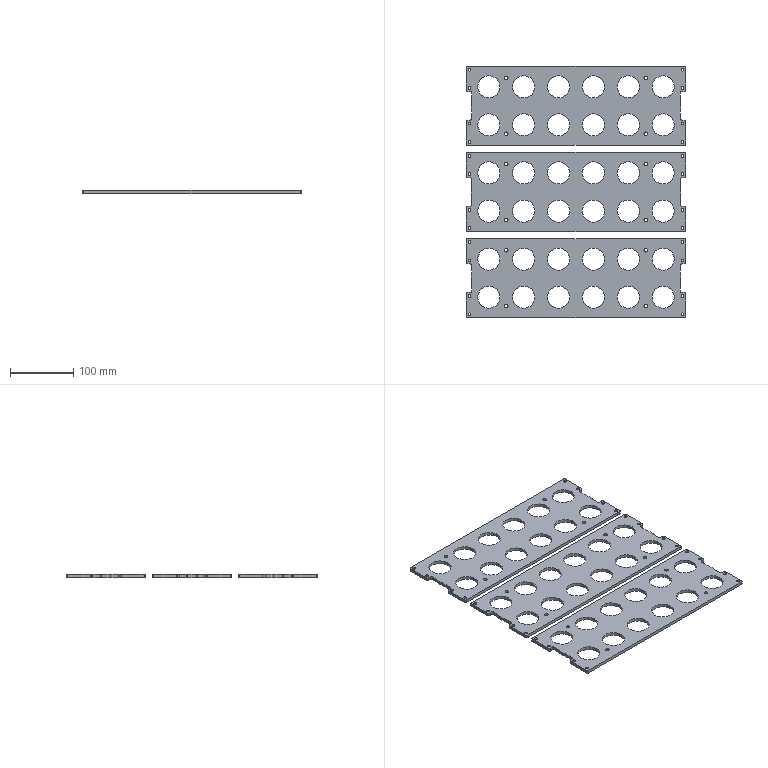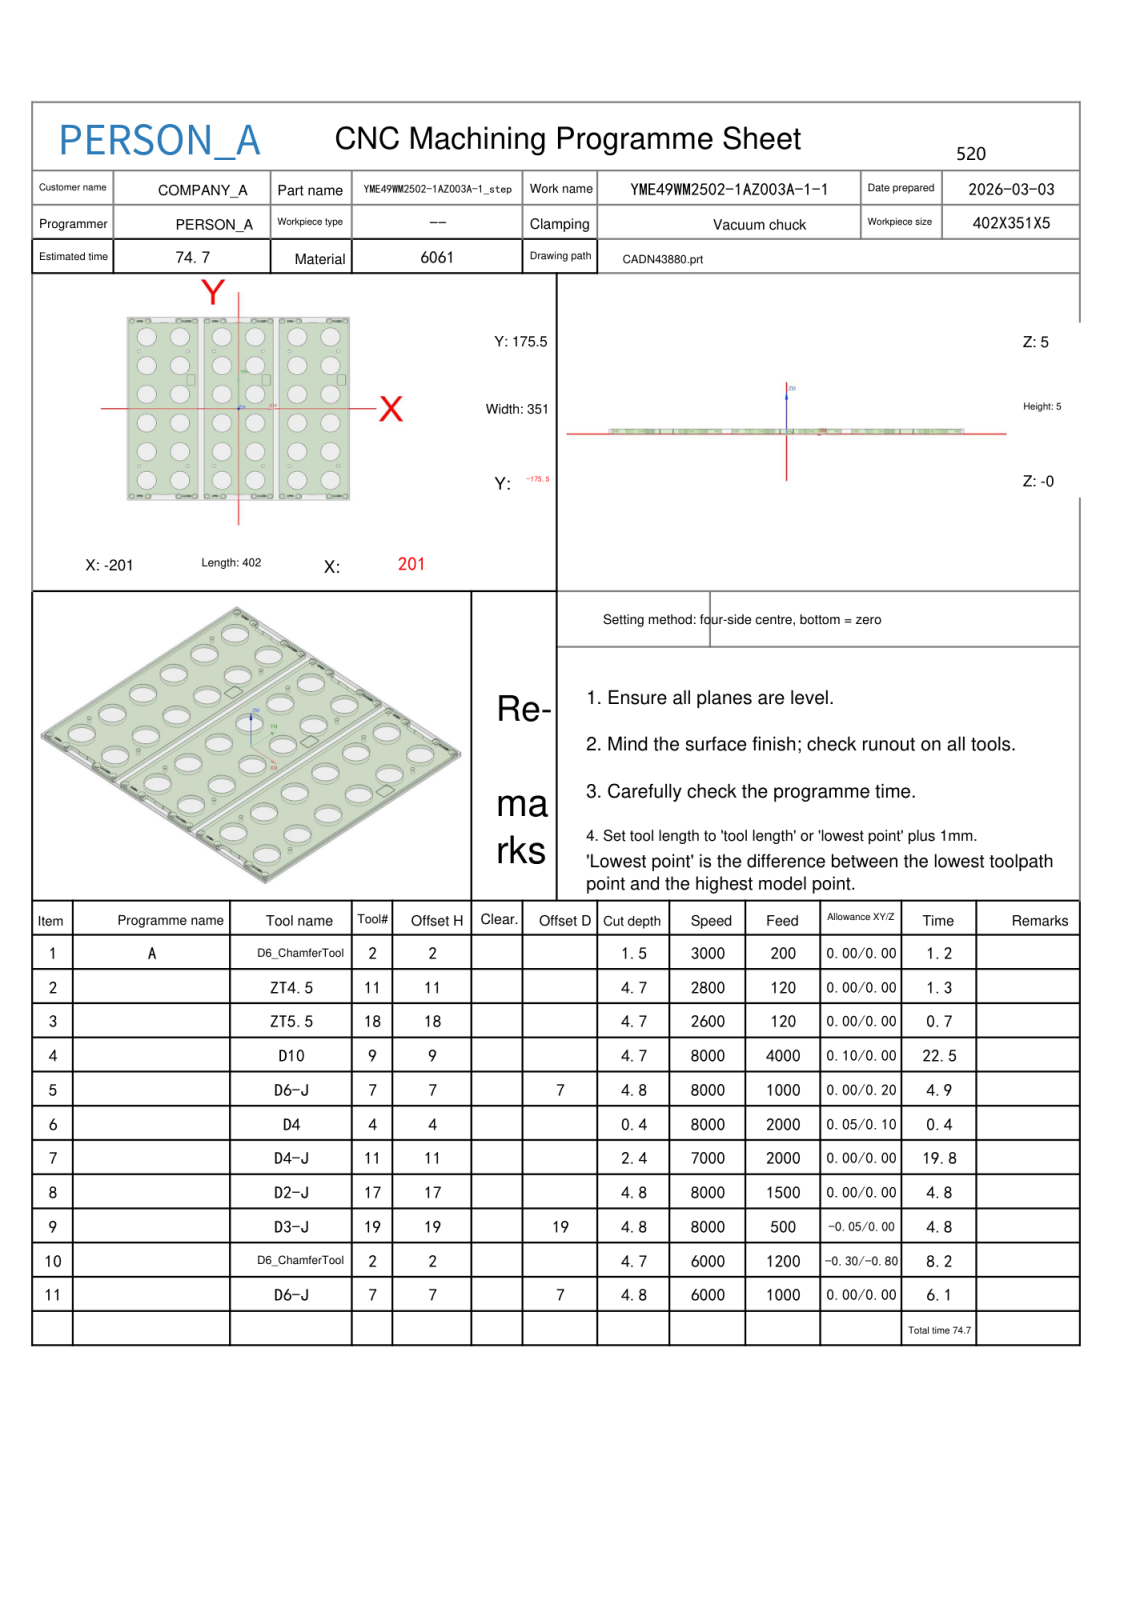NC program | NX | posted by the shop | part box 346 x 397 x 5 mm
Lines 4965 to 5785 of 51232:
N7 T11 M06
(D4-J  D=4. R=0. H=11 ce=0.00 di=0.00)
G00 G90 G54 X-192.342 Y-170.608 M03 S7000
G43 H11 Z35.
M08
Z6.5
G01 X-191.943 Y-170.475 Z6.478 F2000.
X-191.558 Y-170.272 Z6.455
X-191.211 Y-170.01 Z6.432
X-190.91 Y-169.695 Z6.41
X-190.665 Y-169.337 Z6.387
X-190.48 Y-168.943 Z6.364
X-190.384 Y-168.629 Z6.347
X-190.317 Y-168.201 Z6.324
X-190.319 Y-167.767 Z6.301
X-190.367 Y-167.443 Z6.284
X-190.497 Y-167.012 Z6.261
X-190.697 Y-166.608 Z6.237
X-190.961 Y-166.244 Z6.213
X-191.282 Y-165.929 Z6.19
X-191.652 Y-165.671 Z6.166
X-192.059 Y-165.479 Z6.143
X-192.492 Y-165.358 Z6.119
X-192.94 Y-165.31 Z6.095
X-193.389 Y-165.337 Z6.072
X-193.827 Y-165.439 Z6.048
X-194.242 Y-165.613 Z6.025
X-194.523 Y-165.782 Z6.008
X-194.84 Y-166.037 Z5.986
X-195.115 Y-166.337 Z5.965
X-195.342 Y-166.675 Z5.944
X-195.515 Y-167.043 Z5.922
X-195.63 Y-167.433 Z5.901
X-195.686 Y-167.836 Z5.88
Y-168.164 Z5.862
X-195.623 Y-168.601 Z5.839
X-195.49 Y-169.021 Z5.816
X-195.289 Y-169.414 Z5.793
X-195.027 Y-169.769 Z5.77
X-194.711 Y-170.077 Z5.747
X-194.446 Y-170.27 Z5.73
X-194.061 Y-170.473 Z5.707
X-193.649 Y-170.611 Z5.684
X-193.22 Y-170.682 Z5.661
X-192.785 Z5.638
X-192.355 Y-170.613 Z5.616
X-191.943 Y-170.475 Z5.593
X-191.558 Y-170.272 Z5.57
X-191.211 Y-170.01 Z5.547
X-190.91 Y-169.695 Z5.524
X-190.665 Y-169.337 Z5.502
X-190.48 Y-168.943 Z5.479
X-190.384 Y-168.629 Z5.462
X-190.317 Y-168.201 Z5.439
X-190.319 Y-167.767 Z5.416
X-190.367 Y-167.443 Z5.399
X-190.497 Y-167.012 Z5.375
X-190.697 Y-166.608 Z5.352
X-190.961 Y-166.244 Z5.328
X-191.282 Y-165.929 Z5.305
X-191.652 Y-165.671 Z5.281
X-192.059 Y-165.479 Z5.258
X-192.492 Y-165.358 Z5.234
X-192.94 Y-165.31 Z5.21
X-193.389 Y-165.337 Z5.187
X-193.827 Y-165.439 Z5.163
X-194.242 Y-165.613 Z5.14
X-194.523 Y-165.782 Z5.122
X-194.84 Y-166.037 Z5.101
X-195.115 Y-166.337 Z5.08
X-195.342 Y-166.675 Z5.058
X-195.515 Y-167.043 Z5.037
X-195.63 Y-167.433 Z5.016
X-195.686 Y-167.836 Z4.994
Y-168. Z4.986
G03 X-193. Y-170.686 I2.686 J0.0
X-190.314 Y-168. I0.0 J2.686
X-193. Y-165.314 I-2.686 J0.0
X-195.686 Y-168. I0.0 J-2.686
G01 X-195.678 Y-168.08 Z4.979
X-195.667 Y-168.161 Z4.972
G03 X-193. Y-170.672 I2.667 J.161
X-190.328 Y-168. I0.0 J2.672
X-193. Y-165.328 I-2.672 J0.0
X-195.672 Y-168. I0.0 J-2.672
G01 X-195.663 Y-168.08 Z4.965
X-195.653 Y-168.161 Z4.958
G03 X-193. Y-170.658 I2.653 J.161
X-190.342 Y-168. I0.0 J2.658
X-193. Y-165.342 I-2.658 J0.0
X-195.658 Y-168. I0.0 J-2.658
G01 X-195.649 Y-168.08 Z4.951
X-195.639 Y-168.161 Z4.943
G03 X-193. Y-170.643 I2.639 J.161
X-190.357 Y-168. I0.0 J2.643
X-193. Y-165.357 I-2.643 J0.0
X-195.643 Y-168. I0.0 J-2.643
G01 X-195.635 Y-168.08 Z4.936
X-195.624 Y-168.161 Z4.929
G03 X-193. Y-170.629 I2.624 J.161
X-190.371 Y-168. I0.0 J2.629
X-193. Y-165.371 I-2.629 J0.0
X-195.629 Y-168. I0.0 J-2.629
G01 X-195.621 Y-168.08 Z4.922
X-195.61 Y-168.161 Z4.915
G03 X-193. Y-170.615 I2.61 J.161
X-190.385 Y-168. I0.0 J2.615
X-193. Y-165.385 I-2.615 J0.0
X-195.615 Y-168. I0.0 J-2.615
G01 X-195.607 Y-168.08 Z4.908
X-195.596 Y-168.161 Z4.901
G03 X-193. Y-170.601 I2.596 J.161
X-190.399 Y-168. I0.0 J2.601
X-193. Y-165.399 I-2.601 J0.0
X-195.601 Y-168. I0.0 J-2.601
G01 X-195.593 Y-168.08 Z4.894
X-195.582 Y-168.161 Z4.887
G03 X-193. Y-170.587 I2.582 J.161
X-190.413 Y-168. I0.0 J2.587
X-193. Y-165.413 I-2.587 J0.0
X-195.587 Y-168. I0.0 J-2.587
G01 X-195.579 Y-168.08 Z4.88
X-195.568 Y-168.161 Z4.873
G03 X-193. Y-170.573 I2.568 J.161
X-190.427 Y-168. I0.0 J2.573
X-193. Y-165.427 I-2.573 J0.0
X-195.573 Y-168. I0.0 J-2.573
G01 X-195.564 Y-168.08 Z4.866
X-195.554 Y-168.161 Z4.859
G03 X-193. Y-170.559 I2.554 J.161
X-190.441 Y-168. I0.0 J2.559
X-193. Y-165.441 I-2.559 J0.0
X-195.559 Y-168. I0.0 J-2.559
G01 X-195.55 Y-168.08 Z4.852
X-195.539 Y-168.161 Z4.844
G03 X-193. Y-170.544 I2.539 J.161
X-190.456 Y-168. I0.0 J2.544
X-193. Y-165.456 I-2.544 J0.0
X-195.544 Y-168. I0.0 J-2.544
G01 X-195.536 Y-168.08 Z4.837
X-195.525 Y-168.161 Z4.83
G03 X-193. Y-170.53 I2.525 J.161
X-190.47 Y-168. I0.0 J2.53
X-193. Y-165.47 I-2.53 J0.0
X-195.53 Y-168. I0.0 J-2.53
G01 X-195.522 Y-168.08 Z4.823
X-195.511 Y-168.161 Z4.816
G03 X-193. Y-170.516 I2.511 J.161
X-190.484 Y-168. I0.0 J2.516
X-193. Y-165.484 I-2.516 J0.0
X-195.516 Y-168. I0.0 J-2.516
G01 X-195.508 Y-168.08 Z4.809
X-195.497 Y-168.161 Z4.802
G03 X-193. Y-170.503 I2.497 J.161
X-190.498 Y-168. I0.0 J2.502
X-193. Y-165.498 I-2.502 J0.0
X-195.503 Y-168. I0.0 J-2.502
G01 X-195.494 Y-168.08 Z4.795
X-195.483 Y-168.161 Z4.788
G03 X-193. Y-170.488 I2.483 J.161
X-190.512 Y-168. I0.0 J2.488
X-193. Y-165.512 I-2.488 J0.0
X-195.488 Y-168. I0.0 J-2.488
G01 X-195.479 Y-168.08 Z4.781
X-195.469 Y-168.161 Z4.774
G03 X-193. Y-170.474 I2.469 J.161
X-190.526 Y-168. I0.0 J2.474
X-193. Y-165.526 I-2.474 J0.0
X-195.474 Y-168. I0.0 J-2.474
G01 X-195.465 Y-168.08 Z4.767
X-195.454 Y-168.161 Z4.76
G03 X-193. Y-170.46 I2.454 J.161
X-190.54 Y-168. I0.0 J2.46
X-193. Y-165.54 I-2.46 J0.0
X-195.46 Y-168. I0.0 J-2.46
G01 X-195.451 Y-168.08 Z4.753
X-195.44 Y-168.161 Z4.745
G03 X-193. Y-170.445 I2.44 J.161
X-190.555 Y-168. I0.0 J2.445
X-193. Y-165.555 I-2.445 J0.0
X-195.445 Y-168. I0.0 J-2.445
G01 X-195.437 Y-168.08 Z4.738
X-195.426 Y-168.161 Z4.731
G03 X-193. Y-170.431 I2.426 J.161
X-190.569 Y-168. I0.0 J2.431
X-193. Y-165.569 I-2.431 J0.0
X-195.431 Y-168. I0.0 J-2.431
G01 X-195.423 Y-168.08 Z4.724
X-195.412 Y-168.161 Z4.717
G03 X-193. Y-170.417 I2.412 J.161
X-190.583 Y-168. I0.0 J2.417
X-193. Y-165.583 I-2.417 J0.0
X-195.417 Y-168. I0.0 J-2.417
G01 X-195.409 Y-168.08 Z4.71
X-195.398 Y-168.161 Z4.703
G03 X-193. Y-170.403 I2.398 J.161
X-190.597 Y-168. I0.0 J2.403
X-193. Y-165.597 I-2.403 J0.0
X-195.403 Y-168. I0.0 J-2.403
G01 X-195.395 Y-168.08 Z4.696
X-195.383 Y-168.161 Z4.689
G03 X-193. Y-170.389 I2.383 J.161
X-190.611 Y-168. I0.0 J2.389
X-193. Y-165.611 I-2.389 J0.0
X-195.389 Y-168. I0.0 J-2.389
G01 X-195.38 Y-168.08 Z4.682
X-195.369 Y-168.161 Z4.675
G03 X-193. Y-170.375 I2.369 J.161
X-190.625 Y-168. I0.0 J2.375
X-193. Y-165.625 I-2.375 J0.0
X-195.375 Y-168. I0.0 J-2.375
G01 X-195.366 Y-168.08 Z4.668
X-195.355 Y-168.161 Z4.661
G03 X-193. Y-170.361 I2.355 J.161
X-190.639 Y-168. I0.0 J2.361
X-193. Y-165.639 I-2.361 J0.0
X-195.361 Y-168. I0.0 J-2.361
G01 X-195.352 Y-168.08 Z4.654
X-195.341 Y-168.161 Z4.646
G03 X-193. Y-170.346 I2.341 J.161
X-190.654 Y-168. I0.0 J2.346
X-193. Y-165.654 I-2.346 J0.0
X-195.346 Y-168. I0.0 J-2.346
G01 X-195.338 Y-168.08 Z4.639
X-195.327 Y-168.161 Z4.632
G03 X-193. Y-170.332 I2.327 J.161
X-190.668 Y-168. I0.0 J2.332
X-193. Y-165.668 I-2.332 J0.0
X-195.332 Y-168. I0.0 J-2.332
G01 X-195.324 Y-168.08 Z4.625
X-195.313 Y-168.161 Z4.618
G03 X-193. Y-170.318 I2.313 J.161
X-190.682 Y-168. I0.0 J2.318
X-193. Y-165.682 I-2.318 J0.0
X-195.318 Y-168. I0.0 J-2.318
G01 X-195.31 Y-168.08 Z4.611
X-195.298 Y-168.161 Z4.604
G03 X-193. Y-170.304 I2.298 J.161
X-190.696 Y-168. I0.0 J2.304
X-193. Y-165.696 I-2.304 J0.0
X-195.304 Y-168. I0.0 J-2.304
G01 X-195.296 Y-168.08 Z4.597
X-195.284 Y-168.161 Z4.59
G03 X-193. Y-170.29 I2.284 J.161
X-190.71 Y-168. I0.0 J2.29
X-193. Y-165.71 I-2.29 J0.0
X-195.29 Y-168. I0.0 J-2.29
G01 X-195.281 Y-168.08 Z4.583
X-195.27 Y-168.161 Z4.576
G03 X-193. Y-170.276 I2.27 J.161
X-190.724 Y-168. I0.0 J2.276
X-193. Y-165.724 I-2.276 J0.0
X-195.276 Y-168. I0.0 J-2.276
G01 X-195.267 Y-168.08 Z4.569
X-195.256 Y-168.161 Z4.562
G03 X-193. Y-170.262 I2.256 J.161
X-190.738 Y-168. I0.0 J2.262
X-193. Y-165.738 I-2.262 J0.0
X-195.262 Y-168. I0.0 J-2.262
G01 X-195.253 Y-168.08 Z4.555
X-195.242 Y-168.16 Z4.547
G03 X-193. Y-170.247 I2.242 J.16
X-190.753 Y-168. I0.0 J2.247
X-193. Y-165.753 I-2.247 J0.0
X-195.247 Y-168. I0.0 J-2.247
G01 X-195.239 Y-168.08 Z4.54
X-195.228 Y-168.16 Z4.533
G03 X-193. Y-170.233 I2.228 J.16
X-190.767 Y-168. I0.0 J2.233
X-193. Y-165.767 I-2.233 J0.0
X-195.233 Y-168. I0.0 J-2.233
G01 X-195.225 Y-168.08 Z4.526
X-195.213 Y-168.16 Z4.519
G03 X-193. Y-170.219 I2.213 J.16
X-190.781 Y-168. I0.0 J2.219
X-193. Y-165.781 I-2.219 J0.0
X-195.219 Y-168. I0.0 J-2.219
G01 X-195.211 Y-168.08 Z4.512
X-195.199 Y-168.16 Z4.505
G03 X-193. Y-170.205 I2.199 J.16
X-190.795 Y-168. I0.0 J2.205
X-193. Y-165.795 I-2.205 J0.0
X-195.205 Y-168. I0.0 J-2.205
G01 X-195.196 Y-168.08 Z4.498
X-195.185 Y-168.16 Z4.491
G03 X-193. Y-170.191 I2.185 J.16
X-190.809 Y-168. I0.0 J2.191
X-193. Y-165.809 I-2.191 J0.0
X-195.191 Y-168. I0.0 J-2.191
G01 X-195.182 Y-168.08 Z4.484
X-195.171 Y-168.16 Z4.477
G03 X-193. Y-170.177 I2.171 J.16
X-190.823 Y-168. I0.0 J2.177
X-193. Y-165.823 I-2.177 J0.0
X-195.177 Y-168. I0.0 J-2.177
G01 X-195.168 Y-168.08 Z4.47
X-195.157 Y-168.16 Z4.463
G03 X-193. Y-170.163 I2.157 J.16
X-190.837 Y-168. I0.0 J2.163
X-193. Y-165.837 I-2.163 J0.0
X-195.163 Y-168. I0.0 J-2.163
G01 X-195.154 Y-168.08 Z4.456
X-195.142 Y-168.16 Z4.448
G03 X-193. Y-170.148 I2.142 J.16
X-190.852 Y-168. I0.0 J2.148
X-193. Y-165.852 I-2.148 J0.0
X-195.148 Y-168. I0.0 J-2.148
G01 X-195.14 Y-168.08 Z4.441
X-195.128 Y-168.16 Z4.434
G03 X-193. Y-170.134 I2.128 J.16
X-190.866 Y-168. I0.0 J2.134
X-193. Y-165.866 I-2.134 J0.0
X-195.134 Y-168. I0.0 J-2.134
G01 X-195.126 Y-168.08 Z4.427
X-195.114 Y-168.16 Z4.42
G03 X-193. Y-170.12 I2.114 J.16
X-190.88 Y-168. I0.0 J2.12
X-193. Y-165.88 I-2.12 J0.0
X-195.12 Y-168. I0.0 J-2.12
G01 X-195.112 Y-168.08 Z4.413
X-195.1 Y-168.16 Z4.406
G03 X-193. Y-170.106 I2.1 J.16
X-190.894 Y-168. I0.0 J2.106
X-193. Y-165.894 I-2.106 J0.0
X-195.106 Y-168. I0.0 J-2.106
G01 X-195.097 Y-168.08 Z4.399
X-195.086 Y-168.16 Z4.392
G03 X-193. Y-170.092 I2.086 J.16
X-190.908 Y-168. I0.0 J2.092
X-193. Y-165.908 I-2.092 J0.0
X-195.092 Y-168. I0.0 J-2.092
G01 X-195.083 Y-168.08 Z4.385
X-195.072 Y-168.16 Z4.378
G03 X-193. Y-170.078 I2.072 J.16
X-190.922 Y-168. I0.0 J2.078
X-193. Y-165.922 I-2.078 J0.0
X-195.078 Y-168. I0.0 J-2.078
G01 X-195.069 Y-168.08 Z4.371
X-195.057 Y-168.16 Z4.364
G03 X-193. Y-170.064 I2.057 J.16
X-190.936 Y-168. I0.0 J2.064
X-193. Y-165.936 I-2.064 J0.0
X-195.064 Y-168. I0.0 J-2.064
G01 X-195.055 Y-168.08 Z4.357
X-195.043 Y-168.16 Z4.349
G03 X-193. Y-170.049 I2.043 J.16
X-190.951 Y-168. I0.0 J2.049
X-193. Y-165.951 I-2.049 J0.0
X-195.049 Y-168. I0.0 J-2.049
G01 X-195.041 Y-168.08 Z4.342
X-195.029 Y-168.16 Z4.335
G03 X-193. Y-170.035 I2.029 J.16
X-190.965 Y-168. I0.0 J2.035
X-193. Y-165.965 I-2.035 J0.0
X-195.035 Y-168. I0.0 J-2.035
G01 X-195.027 Y-168.08 Z4.328
X-195.015 Y-168.16 Z4.321
G03 X-193. Y-170.021 I2.015 J.16
X-190.979 Y-168. I0.0 J2.021
X-193. Y-165.979 I-2.021 J0.0
X-195.021 Y-168. I0.0 J-2.021
G01 X-195.013 Y-168.08 Z4.314
X-195.001 Y-168.16 Z4.307
G03 X-193. Y-170.007 I2.001 J.16
X-190.993 Y-168. I0.0 J2.007
X-193. Y-165.993 I-2.007 J0.0
X-195.007 Y-168. I0.0 J-2.007
G01 X-194.998 Y-168.08 Z4.3
X-194.986 Y-168.16 Z4.293
G03 X-193. Y-169.993 I1.986 J.16
X-191.007 Y-168. I0.0 J1.993
X-193. Y-166.007 I-1.993 J0.0
X-194.993 Y-168. I0.0 J-1.993
G01 X-194.984 Y-168.08 Z4.286
X-194.972 Y-168.16 Z4.279
G03 X-193. Y-169.979 I1.972 J.16
X-191.021 Y-168. I0.0 J1.979
X-193. Y-166.021 I-1.979 J0.0
X-194.979 Y-168. I0.0 J-1.979
G01 X-194.97 Y-168.08 Z4.272
X-194.958 Y-168.16 Z4.265
G03 X-193. Y-169.965 I1.958 J.16
X-191.035 Y-168. I0.0 J1.965
X-193. Y-166.035 I-1.965 J0.0
X-194.965 Y-168. I0.0 J-1.965
G01 X-194.956 Y-168.08 Z4.258
X-194.944 Y-168.16 Z4.25
G03 X-193. Y-169.95 I1.944 J.16
X-191.05 Y-168. I0.0 J1.95
X-193. Y-166.05 I-1.95 J0.0
X-194.95 Y-168. I0.0 J-1.95
G01 X-194.942 Y-168.08 Z4.243
X-194.93 Y-168.16 Z4.236
G03 X-193. Y-169.936 I1.93 J.16
X-191.064 Y-168. I0.0 J1.936
X-193. Y-166.064 I-1.936 J0.0
X-194.936 Y-168. I0.0 J-1.936
G01 X-194.928 Y-168.08 Z4.229
X-194.915 Y-168.16 Z4.222
G03 X-193. Y-169.922 I1.915 J.16
X-191.078 Y-168. I0.0 J1.922
X-193. Y-166.078 I-1.922 J0.0
X-194.922 Y-168. I0.0 J-1.922
G01 X-194.913 Y-168.08 Z4.215
X-194.901 Y-168.16 Z4.208
G03 X-193. Y-169.908 I1.901 J.16
X-191.092 Y-168. I0.0 J1.908
X-193. Y-166.092 I-1.908 J0.0
X-194.908 Y-168. I0.0 J-1.908
G01 X-194.899 Y-168.08 Z4.201
X-194.887 Y-168.16 Z4.194
G03 X-193. Y-169.894 I1.887 J.16
X-191.106 Y-168. I0.0 J1.894
X-193. Y-166.106 I-1.894 J0.0
X-194.894 Y-168. I0.0 J-1.894
G01 X-194.885 Y-168.08 Z4.187
X-194.873 Y-168.16 Z4.18
G03 X-193. Y-169.88 I1.873 J.16
X-191.12 Y-168. I0.0 J1.88
X-193. Y-166.12 I-1.88 J0.0
X-194.88 Y-168. I0.0 J-1.88
G01 X-194.871 Y-168.08 Z4.173
X-194.859 Y-168.16 Z4.166
G03 X-193. Y-169.866 I1.859 J.16
X-191.134 Y-168. I0.0 J1.866
X-193. Y-166.134 I-1.866 J0.0
X-194.866 Y-168. I0.0 J-1.866
G01 X-194.857 Y-168.08 Z4.159
X-194.845 Y-168.16 Z4.151
G03 X-193. Y-169.851 I1.845 J.16
X-191.149 Y-168. I0.0 J1.851
X-193. Y-166.149 I-1.851 J0.0
X-194.851 Y-168. I0.0 J-1.851
G01 X-194.843 Y-168.08 Z4.144
X-194.83 Y-168.16 Z4.137
G03 X-193. Y-169.837 I1.83 J.16
X-191.163 Y-168. I0.0 J1.837
X-193. Y-166.163 I-1.837 J0.0
X-194.837 Y-168. I0.0 J-1.837
G01 X-194.829 Y-168.08 Z4.13
X-194.816 Y-168.16 Z4.123
G03 X-193. Y-169.823 I1.816 J.16
X-191.177 Y-168. I0.0 J1.823
X-193. Y-166.177 I-1.823 J0.0
X-194.823 Y-168. I0.0 J-1.823
G01 X-194.814 Y-168.08 Z4.116
X-194.802 Y-168.16 Z4.109
G03 X-193. Y-169.809 I1.802 J.16
X-191.191 Y-168. I0.0 J1.809
X-193. Y-166.191 I-1.809 J0.0
X-194.809 Y-168. I0.0 J-1.809
G01 X-194.8 Y-168.08 Z4.102
X-194.788 Y-168.16 Z4.095
G03 X-193. Y-169.795 I1.788 J.16
X-191.205 Y-168. I0.0 J1.795
X-193. Y-166.205 I-1.795 J0.0
X-194.795 Y-168. I0.0 J-1.795
G01 X-194.786 Y-168.08 Z4.088
X-194.774 Y-168.16 Z4.081
G03 X-193. Y-169.781 I1.774 J.16
X-191.219 Y-168. I0.0 J1.781
X-193. Y-166.219 I-1.781 J0.0
X-194.781 Y-168. I0.0 J-1.781
G01 X-194.772 Y-168.08 Z4.074
X-194.759 Y-168.16 Z4.067
G03 X-193. Y-169.767 I1.759 J.16
X-191.233 Y-168. I0.0 J1.767
X-193. Y-166.233 I-1.767 J0.0
X-194.767 Y-168. I0.0 J-1.767
G01 X-194.758 Y-168.08 Z4.06
X-194.745 Y-168.16 Z4.052
G03 X-193. Y-169.752 I1.745 J.16
X-191.248 Y-168. I0.0 J1.752
X-193. Y-166.248 I-1.752 J0.0
X-194.752 Y-168. I0.0 J-1.752
G01 X-194.744 Y-168.08 Z4.045
X-194.731 Y-168.16 Z4.038
G03 X-193. Y-169.738 I1.731 J.16
X-191.262 Y-168. I0.0 J1.738
X-193. Y-166.262 I-1.738 J0.0
X-194.738 Y-168. I0.0 J-1.738
G01 X-194.729 Y-168.08 Z4.031
X-194.717 Y-168.16 Z4.024
G03 X-193. Y-169.724 I1.717 J.16
X-191.276 Y-168. I0.0 J1.724
X-193. Y-166.276 I-1.724 J0.0
X-194.724 Y-168. I0.0 J-1.724
G01 X-194.715 Y-168.08 Z4.017
X-194.703 Y-168.16 Z4.01
G03 X-193. Y-169.71 I1.703 J.16
X-191.29 Y-168. I0.0 J1.71
X-193. Y-166.29 I-1.71 J0.0
X-194.71 Y-168. I0.0 J-1.71
G01 X-194.701 Y-168.08 Z4.003
X-194.688 Y-168.16 Z3.996
G03 X-193. Y-169.696 I1.688 J.16
X-191.304 Y-168. I0.0 J1.696
X-193. Y-166.304 I-1.696 J0.0
X-194.696 Y-168. I0.0 J-1.696
G01 X-194.687 Y-168.08 Z3.989
X-194.674 Y-168.16 Z3.982
G03 X-193. Y-169.682 I1.674 J.16
X-191.318 Y-168. I0.0 J1.682
X-193. Y-166.318 I-1.682 J0.0
X-194.682 Y-168. I0.0 J-1.682
G01 X-194.673 Y-168.08 Z3.975
X-194.66 Y-168.16 Z3.968
G03 X-193. Y-169.668 I1.66 J.16
X-191.332 Y-168. I0.0 J1.668
X-193. Y-166.332 I-1.668 J0.0
X-194.668 Y-168. I0.0 J-1.668
G01 X-194.659 Y-168.08 Z3.961
X-194.646 Y-168.16 Z3.953
G03 X-193. Y-169.653 I1.646 J.16
X-191.347 Y-168. I0.0 J1.653
X-193. Y-166.347 I-1.653 J0.0
X-194.653 Y-168. I0.0 J-1.653
G01 X-194.644 Y-168.08 Z3.946
X-194.632 Y-168.16 Z3.939
G03 X-193. Y-169.639 I1.632 J.16
X-191.361 Y-168. I0.0 J1.639
X-193. Y-166.361 I-1.639 J0.0
X-194.639 Y-168. I0.0 J-1.639
G01 X-194.63 Y-168.08 Z3.932
X-194.617 Y-168.16 Z3.925
G03 X-193. Y-169.625 I1.617 J.16
X-191.375 Y-168. I0.0 J1.625
X-193. Y-166.375 I-1.625 J0.0
X-194.625 Y-168. I0.0 J-1.625
G01 X-194.616 Y-168.08 Z3.918
X-194.603 Y-168.16 Z3.911
G03 X-193. Y-169.611 I1.603 J.16
X-191.389 Y-168. I0.0 J1.611
X-193. Y-166.389 I-1.611 J0.0
X-194.611 Y-168. I0.0 J-1.611
G01 X-194.602 Y-168.08 Z3.904
X-194.589 Y-168.16 Z3.897
G03 X-193. Y-169.597 I1.589 J.16
X-191.403 Y-168. I0.0 J1.597
X-193. Y-166.403 I-1.597 J0.0
X-194.597 Y-168. I0.0 J-1.597
G01 X-194.588 Y-168.08 Z3.89
X-194.575 Y-168.16 Z3.883
G03 X-193. Y-169.583 I1.575 J.16
X-191.417 Y-168. I0.0 J1.583
X-193. Y-166.417 I-1.583 J0.0
X-194.583 Y-168. I0.0 J-1.583
G01 X-194.574 Y-168.08 Z3.876
X-194.56 Y-168.16 Z3.869
G03 X-193. Y-169.569 I1.56 J.16
X-191.431 Y-168. I0.0 J1.569
X-193. Y-166.431 I-1.569 J0.0
X-194.569 Y-168. I0.0 J-1.569
G01 X-194.56 Y-168.08 Z3.862
X-194.546 Y-168.16 Z3.854
G03 X-193. Y-169.554 I1.546 J.16
X-191.446 Y-168. I0.0 J1.554
X-193. Y-166.446 I-1.554 J0.0
X-194.554 Y-168. I0.0 J-1.554
G01 X-194.545 Y-168.08 Z3.847
X-194.532 Y-168.16 Z3.84
G03 X-193. Y-169.54 I1.532 J.16
X-191.46 Y-168. I0.0 J1.54
X-193. Y-166.46 I-1.54 J0.0
X-194.54 Y-168. I0.0 J-1.54
G01 X-194.531 Y-168.08 Z3.833
X-194.518 Y-168.16 Z3.826
G03 X-193. Y-169.526 I1.518 J.16
X-191.474 Y-168. I0.0 J1.526
X-193. Y-166.474 I-1.526 J0.0
X-194.526 Y-168. I0.0 J-1.526
G01 X-194.517 Y-168.08 Z3.819
X-194.504 Y-168.16 Z3.812
G03 X-193. Y-169.512 I1.504 J.16
X-191.488 Y-168. I0.0 J1.512
X-193. Y-166.488 I-1.512 J0.0
X-194.512 Y-168. I0.0 J-1.512
G01 X-194.503 Y-168.08 Z3.805
X-194.489 Y-168.16 Z3.798
G03 X-193. Y-169.498 I1.489 J.16
X-191.502 Y-168. I0.0 J1.498
X-193. Y-166.502 I-1.498 J0.0
X-194.498 Y-168. I0.0 J-1.498
G01 X-194.489 Y-168.08 Z3.791
X-194.475 Y-168.16 Z3.784
G03 X-193. Y-169.484 I1.475 J.16
X-191.516 Y-168. I0.0 J1.484
X-193. Y-166.516 I-1.484 J0.0
X-194.484 Y-168. I0.0 J-1.484
G01 X-194.475 Y-168.08 Z3.777
X-194.461 Y-168.16 Z3.77
G03 X-193. Y-169.47 I1.461 J.16
X-191.53 Y-168. I0.0 J1.47
X-193. Y-166.53 I-1.47 J0.0
X-194.47 Y-168. I0.0 J-1.47
G01 X-194.46 Y-168.08 Z3.763
X-194.447 Y-168.16 Z3.755
G03 X-193. Y-169.455 I1.447 J.16
X-191.545 Y-168. I0.0 J1.455
X-193. Y-166.545 I-1.455 J0.0
X-194.455 Y-168. I0.0 J-1.455
G01 X-194.446 Y-168.08 Z3.748
X-194.432 Y-168.16 Z3.741
G03 X-193. Y-169.441 I1.432 J.16
X-191.559 Y-168. I0.0 J1.441
X-193. Y-166.559 I-1.441 J0.0
X-194.441 Y-168. I0.0 J-1.441
G01 X-194.432 Y-168.08 Z3.734
X-194.418 Y-168.16 Z3.727
G03 X-193. Y-169.427 I1.418 J.16
X-191.573 Y-168. I0.0 J1.427
X-193. Y-166.573 I-1.427 J0.0
X-194.427 Y-168. I0.0 J-1.427
G01 X-194.418 Y-168.08 Z3.72
X-194.404 Y-168.16 Z3.713
G03 X-193. Y-169.413 I1.404 J.16
X-191.587 Y-168. I0.0 J1.413
X-193. Y-166.587 I-1.413 J0.0
X-194.413 Y-168. I0.0 J-1.413
G01 X-194.404 Y-168.08 Z3.706
X-194.39 Y-168.16 Z3.699
G03 X-193. Y-169.399 I1.39 J.16
X-191.601 Y-168. I0.0 J1.399
X-193. Y-166.601 I-1.399 J0.0
X-194.399 Y-168. I0.0 J-1.399
G01 X-194.39 Y-168.08 Z3.692
X-194.376 Y-168.16 Z3.685
G03 X-193. Y-169.385 I1.376 J.16
X-191.615 Y-168. I0.0 J1.385
X-193. Y-166.615 I-1.385 J0.0
X-194.385 Y-168. I0.0 J-1.385
G01 X-194.375 Y-168.08 Z3.678
X-194.361 Y-168.16 Z3.671
G03 X-193. Y-169.371 I1.361 J.16
X-191.629 Y-168. I0.0 J1.371
X-193. Y-166.629 I-1.371 J0.0
X-194.371 Y-168. I0.0 J-1.371
G01 X-194.361 Y-168.08 Z3.664
X-194.347 Y-168.16 Z3.656
G03 X-193. Y-169.356 I1.347 J.16
X-191.644 Y-168. I0.0 J1.356
X-193. Y-166.644 I-1.356 J0.0
X-194.356 Y-168. I0.0 J-1.356
G01 X-194.347 Y-168.08 Z3.649
X-194.333 Y-168.16 Z3.642
G03 X-193. Y-169.342 I1.333 J.16
X-191.658 Y-168. I0.0 J1.342
X-193. Y-166.658 I-1.342 J0.0
X-194.342 Y-168. I0.0 J-1.342
G01 X-194.333 Y-168.08 Z3.635
X-194.319 Y-168.16 Z3.628
G03 X-193. Y-169.328 I1.319 J.16
X-191.672 Y-168. I0.0 J1.328
X-193. Y-166.672 I-1.328 J0.0
X-194.328 Y-168. I0.0 J-1.328
G01 X-194.319 Y-168.08 Z3.621
X-194.304 Y-168.16 Z3.614
G03 X-193. Y-169.314 I1.304 J.16
X-191.686 Y-168. I0.0 J1.314
X-193. Y-166.686 I-1.314 J0.0
X-194.314 Y-168. I0.0 J-1.314
G01 X-194.305 Y-168.08 Z3.607
X-194.29 Y-168.16 Z3.6
G03 X-193. Y-169.3 I1.29 J.16
X-191.7 Y-168. I0.0 J1.3
X-193. Y-166.7 I-1.3 J0.0
X-194.3 Y-168. I0.0 J-1.3
G01 X-194.29 Y-168.08 Z3.593
X-194.276 Y-168.159 Z3.586
G03 X-193. Y-169.286 I1.276 J.159
X-191.714 Y-168. I0.0 J1.286
X-193. Y-166.714 I-1.286 J0.0
X-194.286 Y-168. I0.0 J-1.286
G01 X-194.276 Y-168.08 Z3.579
X-194.262 Y-168.159 Z3.572
G03 X-193. Y-169.272 I1.262 J.159
X-191.728 Y-168. I0.0 J1.272
X-193. Y-166.728 I-1.272 J0.0
X-194.272 Y-168. I0.0 J-1.272
G01 X-194.262 Y-168.08 Z3.565
X-194.247 Y-168.159 Z3.558
G03 X-193. Y-169.258 I1.247 J.159
X-191.742 Y-168. I0.0 J1.258
X-193. Y-166.742 I-1.258 J0.0
X-194.258 Y-168. I0.0 J-1.258
G01 X-194.248 Y-168.08 Z3.55
X-194.233 Y-168.159 Z3.543
G03 X-193. Y-169.243 I1.233 J.159
X-191.757 Y-168. I0.0 J1.243
X-193. Y-166.757 I-1.243 J0.0
X-194.243 Y-168. I0.0 J-1.243
G01 X-194.234 Y-168.08 Z3.536
X-194.219 Y-168.159 Z3.529
G03 X-193. Y-169.229 I1.219 J.159
X-191.771 Y-168. I0.0 J1.229
X-193. Y-166.771 I-1.229 J0.0
X-194.229 Y-168. I0.0 J-1.229
G01 X-194.22 Y-168.08 Z3.522
X-194.205 Y-168.159 Z3.515
G03 X-193. Y-169.215 I1.205 J.159
X-191.785 Y-168. I0.0 J1.215
X-193. Y-166.785 I-1.215 J0.0
X-194.215 Y-168. I0.0 J-1.215
G01 X-194.205 Y-168.08 Z3.508
X-194.19 Y-168.159 Z3.501
G03 X-193. Y-169.201 I1.19 J.159
X-191.799 Y-168. I0.0 J1.201
X-193. Y-166.799 I-1.201 J0.0
X-194.201 Y-168. I0.0 J-1.201
G01 X-194.191 Y-168.08 Z3.494
X-194.176 Y-168.159 Z3.487
G03 X-193. Y-169.187 I1.176 J.159
X-191.813 Y-168. I0.0 J1.187
X-193. Y-166.813 I-1.187 J0.0
X-194.187 Y-168. I0.0 J-1.187
G01 X-194.177 Y-168.08 Z3.48
X-194.162 Y-168.159 Z3.473
G03 X-193. Y-169.173 I1.162 J.159
X-191.827 Y-168. I0.0 J1.173
X-193. Y-166.827 I-1.173 J0.0
X-194.173 Y-168. I0.0 J-1.173
G01 X-194.163 Y-168.08 Z3.466
X-194.148 Y-168.159 Z3.459
G03 X-193. Y-169.159 I1.148 J.159
X-191.841 Y-168. I0.0 J1.159
X-193. Y-166.841 I-1.159 J0.0
X-194.159 Y-168. I0.0 J-1.159
G01 X-194.149 Y-168.08 Z3.451
X-194.133 Y-168.159 Z3.444
G03 X-193. Y-169.144 I1.133 J.159
X-191.856 Y-168. I0.0 J1.144
X-193. Y-166.856 I-1.144 J0.0
X-194.144 Y-168. I0.0 J-1.144
G01 X-194.134 Y-168.08 Z3.437
X-194.119 Y-168.159 Z3.43
G03 X-193. Y-169.13 I1.119 J.159
X-191.87 Y-168. I0.0 J1.13
X-193. Y-166.87 I-1.13 J0.0
X-194.13 Y-168. I0.0 J-1.13
G01 X-194.12 Y-168.08 Z3.423
X-194.105 Y-168.159 Z3.416
G03 X-193. Y-169.116 I1.105 J.159
X-191.884 Y-168. I0.0 J1.116
X-193. Y-166.884 I-1.116 J0.0
X-194.116 Y-168. I0.0 J-1.116
G01 X-194.106 Y-168.08 Z3.409
X-194.09 Y-168.159 Z3.402
G03 X-193. Y-169.102 I1.09 J.159
X-191.898 Y-168. I0.0 J1.102
X-193. Y-166.898 I-1.102 J0.0
X-194.102 Y-168. I0.0 J-1.102
G01 X-194.092 Y-168.08 Z3.395
X-194.076 Y-168.159 Z3.388
G03 X-193. Y-169.088 I1.076 J.159
X-191.912 Y-168. I0.0 J1.088
X-193. Y-166.912 I-1.088 J0.0
X-194.088 Y-168. I0.0 J-1.088
G01 X-194.078 Y-168.08 Z3.381
X-194.062 Y-168.159 Z3.374
G03 X-193. Y-169.074 I1.062 J.159
X-191.926 Y-168. I0.0 J1.074
X-193. Y-166.926 I-1.074 J0.0
X-194.074 Y-168. I0.0 J-1.074
G01 X-194.064 Y-168.08 Z3.367
X-194.048 Y-168.159 Z3.36
G03 X-193. Y-169.06 I1.048 J.159
X-191.94 Y-168. I0.0 J1.06
X-193. Y-166.94 I-1.06 J0.0
X-194.06 Y-168. I0.0 J-1.06
G01 X-194.049 Y-168.08 Z3.352
X-194.033 Y-168.159 Z3.345
G03 X-193. Y-169.045 I1.033 J.159
X-191.955 Y-168. I0.0 J1.045
X-193. Y-166.955 I-1.045 J0.0
X-194.045 Y-168. I0.0 J-1.045
G01 X-194.035 Y-168.08 Z3.338
X-194.019 Y-168.159 Z3.331
G03 X-193. Y-169.031 I1.019 J.159
X-191.969 Y-168. I0.0 J1.031
X-193. Y-166.969 I-1.031 J0.0
X-194.031 Y-168. I0.0 J-1.031
G01 X-194.021 Y-168.08 Z3.324
X-194.005 Y-168.159 Z3.317
G03 X-193. Y-169.017 I1.005 J.159
X-191.983 Y-168. I0.0 J1.017
X-193. Y-166.983 I-1.017 J0.0
X-194.017 Y-168. I0.0 J-1.017
G01 X-194.007 Y-168.08 Z3.31
X-193.99 Y-168.159 Z3.303
G03 X-193. Y-169.003 I.99 J.159
X-191.997 Y-168. I0.0 J1.003
X-193. Y-166.997 I-1.003 J0.0
X-194.003 Y-168. I0.0 J-1.003
G01 X-193.993 Y-168.08 Z3.296
X-193.976 Y-168.159 Z3.289
G03 X-193. Y-168.989 I.976 J.159
X-192.011 Y-168. I0.0 J.989
X-193. Y-167.011 I-.989 J0.0
X-193.989 Y-168. I0.0 J-.989
G01 X-193.979 Y-168.08 Z3.282
X-193.962 Y-168.159 Z3.275
G03 X-193. Y-168.975 I.962 J.159
X-192.025 Y-168. I0.0 J.975
X-193. Y-167.025 I-.975 J0.0
X-193.975 Y-168. I0.0 J-.975
G01 X-193.964 Y-168.08 Z3.268
X-193.947 Y-168.159 Z3.261
G03 X-193. Y-168.961 I.947 J.159
X-192.039 Y-168. I0.0 J.961
X-193. Y-167.039 I-.961 J0.0
X-193.961 Y-168. I0.0 J-.961
G01 X-193.95 Y-168.08 Z3.253
X-193.933 Y-168.159 Z3.246
G03 X-193. Y-168.946 I.933 J.159
X-192.054 Y-168. I0.0 J.946
X-193. Y-167.054 I-.946 J0.0
X-193.946 Y-168. I0.0 J-.946
G01 X-193.936 Y-168.08 Z3.239
X-193.919 Y-168.158 Z3.232
G03 X-193. Y-168.932 I.919 J.158
X-192.068 Y-168. I0.0 J.932